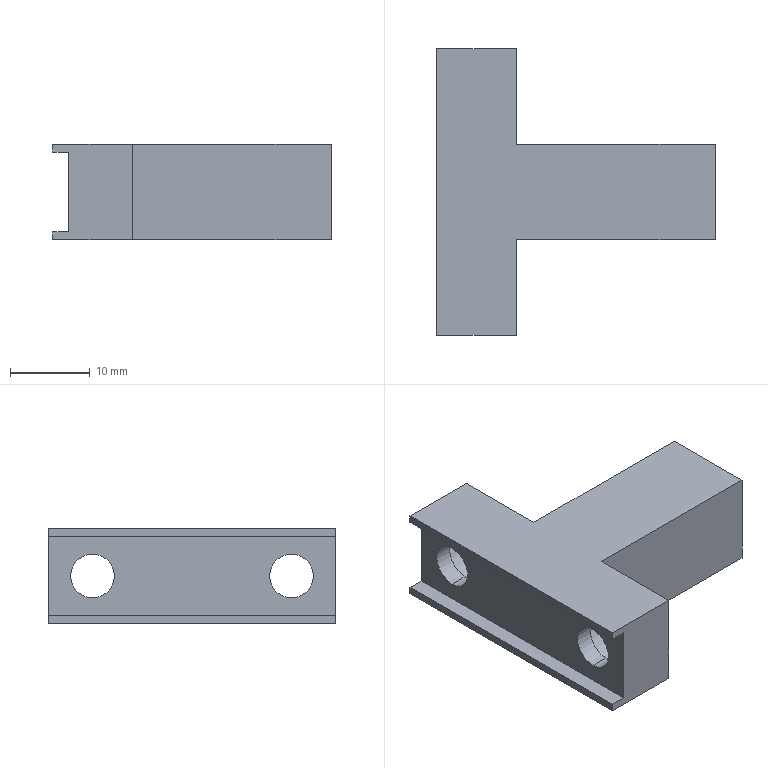Part | STEP file | PN_0024 | 1 solid | 24 faces | box 35 x 36 x 12 mm | volume 6195 mm3 | plane 16 | cylinder 8 | commonest cylinder face diameters 5.5 x4 10 x4